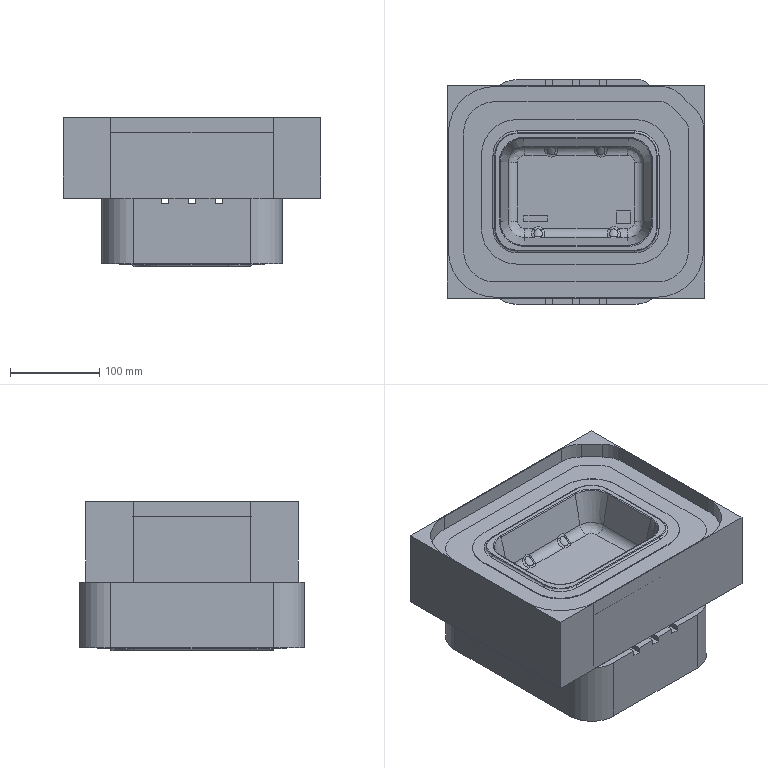NC program | NX | posted with a generic post | part box 287.436 x 251.436 x 167.016 mm
Lines 9781 to 10739 of 118587:
(02 , TOOL : D8)
N19560 M6
N19562 G53
N19564 G17 G0 G90 X-74.765 Y-30.868 S7000 M3 M8
N19566 G43 Z240.5 H0
N19568 Z77.049
N19570 G94 G1 Z76.049 F4500.
N19572 X-78.947
N19574 G3 X-80.547 Y-32.468 R1.6
N19576 G1 Y-33.767
N19578 G3 X-74.266 Y-49.06 R21.919
N19580 X-58.521 Y-55.793 R21.988
N19582 G1 X58.521
N19584 G3 X74.265 Y-49.06 R21.985
N19586 X80.547 Y-33.767 R21.921
N19588 G1 Y-32.476
N19590 G3 X78.947 Y-30.876 R1.6
N19592 G1 X74.765
N19594 Z77.049
N19596 G0 Z93.5
N19598 X43.464 Y-40.046
N19600 Z38.027
N19602 G1 Z37.027
N19604 X44.625 Y-43.436
N19606 G3 X46.657 Y-44.431 R1.6
N19608 G2 X48.138 Y-44.506 R2.
N19610 G3 X48.699 Y-44.666 R1.921
N19612 G2 X50.449 Y-46.65 R2.
N19614 G1 X48.385
N19616 G2 X47.261 Y-46.296 R2.232
N19618 G3 X45.531 Y-45.398 R8.895
N19620 G2 X46.657 Y-44.431 R2.
N19622 G3 X47.652 Y-42.399 R1.6
N19624 G1 X46.678 Y-39.553
N19626 Z38.027
N19628 G0 Z79.049
N19630 X46.793 Y-39.422
N19632 Z37.677
N19634 G1 Z36.677
N19636 X45.177 Y-43.03
N19638 G3 X45.983 Y-45.144 R1.6
N19640 G2 X47.694 Y-46.153 R8.929
N19642 G1 X47.896 Y-46.296
N19644 G3 X48.52 Y-46.517 R1.08
N19646 G1 X50.875
N19648 G3 X52.475 Y-44.917 R1.6
N19650 G1 Y-40.749
N19652 Z37.677
N19654 G0 Z40.027
N19656 X47.461 Y-39.221
N19658 Z37.328
N19660 G1 Z36.328
N19662 X45.678 Y-42.766
N19664 G3 X46.388 Y-44.914 R1.6
N19666 G2 X48.415 Y-46.28 R9.634
N19668 G3 X48.653 Y-46.37 R0.361
N19670 G1 X51.271
N19672 G3 X52.871 Y-44.77 R1.6
N19674 G1 Y-40.601
N19676 Z37.328
N19678 G0 Z39.677
N19680 X48.003 Y-39.005
N19682 Z36.978
N19684 G1 Z35.978
N19686 X46.099 Y-42.475
N19688 G3 X46.732 Y-44.647 R1.6
N19690 G2 X48.81 Y-46.207 R9.174
N19692 G1 X51.593
N19694 G3 X53.193 Y-44.607 R1.6
N19696 G1 Y-40.439
N19698 Z36.978
N19700 G0 Z39.328
N19702 X45.53 Y-38.647
N19704 Z36.629
N19706 G1 Z35.629
N19708 X46.311 Y-42.373
N19710 G3 X48.205 Y-43.611 R1.6
N19712 G2 X49.606 Y-43.831 R2.
N19714 G3 X50.237 Y-44.056 R1.921
N19716 G2 X51.905 Y-46.028 R2.
N19718 G1 X49.081
N19720 G3 X47.011 Y-44.375 R9.539
N19722 G2 X48.205 Y-43.611 R2.
N19724 G3 X49.443 Y-41.717 R1.6
N19726 G1 X48.826 Y-38.772
N19728 Z36.629
N19730 G0 Z38.978
N19732 X44.496 Y-38.001
N19734 Z36.279
N19736 G1 Z35.279
N19738 X46.096 Y-42.468
N19740 G3 X48.142 Y-43.434 R1.6
N19742 G2 X49.857 Y-43.609 R2.
N19744 G3 X50.528 Y-43.861 R1.921
N19746 G2 X52.186 Y-45.832 R2.
N19748 G1 X49.308
N19750 G3 X47.244 Y-44.081 R9.592
N19752 G2 X48.142 Y-43.434 R2.
N19754 G3 X49.108 Y-41.388 R1.6
N19756 G1 X48.094 Y-38.556
N19758 Z36.279
N19760 G0 Z38.629
N19762 X44.067 Y-37.505
N19764 Z35.929
N19766 G1 Z34.929
N19768 X46.989 Y-42.975
N19770 G3 X48.072 Y-43.303 R0.8
N19772 G2 X50.085 Y-43.378 R2.
N19774 G3 X50.78 Y-43.647 R1.921
N19776 G2 X52.432 Y-45.617 R2.
N19778 G1 X49.518
N19780 G3 X47.47 Y-43.797 R9.774
N19782 G2 X48.072 Y-43.303 R2.
N19784 G3 X48.729 Y-41.138 R1.6
N19786 G1 X47.217 Y-38.308
N19788 Z35.929
N19790 G0 Z38.279
N19792 X52.424 Y-38.815
N19794 Z35.58
N19796 G1 Z34.58
N19798 X50.22 Y-43.513
N19800 G3 X47.981 Y-43.182 R1.6
N19802 G2 X50.28 Y-43.121 R2.
N19804 G3 X51.008 Y-43.412 R1.921
N19806 G2 X52.659 Y-45.382 R2.
N19808 G1 X49.691
N19810 G3 X47.659 Y-43.482 R9.75
N19812 G2 X47.981 Y-43.182 R2.
N19814 G3 X48.312 Y-40.943 R1.6
N19816 G1 X45.665 Y-37.378
N19818 Z35.58
N19820 G0 Z37.929
N19822 X50.066 Y-37.705
N19824 Z35.23
N19826 G1 Z34.23
N19828 X47.589 Y-41.031
N19830 G3 X47.916 Y-43.27 R1.6
N19832 X47.745 Y-43.145 R10.561
N19834 G2 X50.415 Y-42.827 R2.
N19836 G3 X51.2 Y-43.155 R1.921
N19838 G2 X52.856 Y-45.125 R2.
N19840 G1 X49.84
N19842 G3 X47.916 Y-43.27 R10.561
N19844 X50.155 Y-42.943 R1.6
N19846 G1 X53.266 Y-38.766
N19848 Z35.23
N19850 G0 Z37.58
N19852 X50.463 Y-37.426
N19854 Z34.881
N19856 G1 Z33.881
N19858 X47.857 Y-40.751
N19860 G3 X48.129 Y-42.998 R1.6
N19862 X47.874 Y-42.804 R10.553
N19864 G2 X50.55 Y-42.526 R2.
N19866 G3 X51.37 Y-42.872 R1.921
N19868 G2 X53.038 Y-44.845 R2.
N19870 G1 X49.965
N19872 G3 X48.129 Y-42.998 R10.553
N19874 X50.375 Y-42.725 R1.6
N19876 G1 X53.639 Y-38.562
N19878 Z34.881
N19880 G0 Z37.23
N19882 X50.071 Y-37.028
N19884 Z34.531
N19886 G1 Z33.531
N19888 X47.67 Y-40.209
N19890 G3 X47.983 Y-42.45 R1.6
N19892 G2 X50.067 Y-44.538 R10.607
N19894 G1 X53.204
N19896 G3 X54.804 Y-42.938 R1.6
N19898 G1 Y-38.769
N19900 Z34.531
N19902 G0 Z36.881
N19904 X50.047 Y-36.563
N19906 Z34.182
N19908 G1 Z33.182
N19910 X47.645 Y-39.711
N19912 G3 X47.946 Y-41.954 R1.6
N19914 G2 X48.955 Y-42.841 R9.628
N19916 G1 X49.077 Y-42.963
N19918 X50.147 Y-44.201
N19920 X53.365
N19922 G3 X54.965 Y-42.601 R1.6
N19924 G1 Y-38.432
N19926 Z34.182
N19928 G0 Z36.531
N19930 X47.442 Y-35.763
N19932 Z33.832
N19934 G1 Z32.832
N19936 X47.658 Y-39.461
N19938 G3 X49.348 Y-40.965 R1.6
N19940 G2 X50.734 Y-41.415 R2.
N19942 G3 X51.752 Y-41.841 R1.921
N19944 G2 X53.544 Y-43.83 R2.
N19946 G1 X50.204
N19948 X49.363 Y-42.841
N19950 G3 X48.025 Y-41.574 R9.605
N19952 G2 X49.348 Y-40.965 R2.
N19954 G3 X50.852 Y-39.274 R1.6
N19956 G1 X50.677 Y-36.27
N19958 Z33.832
N19960 G0 Z79.049
N19962 X37.967 Y-39.545
N19964 Z38.027
N19966 G1 Z37.027
N19968 X36.996 Y-42.393
N19970 G3 X37.995 Y-44.423 R1.6
N19972 G2 X39.124 Y-45.393 R2.
N19974 G3 X37.381 Y-46.296 R8.895
N19976 G2 X36.243 Y-46.65 R2.116
N19978 G1 X34.19
N19980 G2 X35.941 Y-44.665 R2.
N19982 G3 X36.509 Y-44.502 R1.921
N19984 G2 X37.995 Y-44.423 R2.
N19986 G3 X40.026 Y-43.425 R1.6
N19988 G1 X41.176 Y-40.047
N19990 Z38.027
N19992 G0 Z79.049
N19994 X32.166 Y-40.749
N19996 Z37.677
N19998 G1 Z36.677
N20000 Y-44.917
N20002 G3 X33.766 Y-46.517 R1.6
N20004 G1 X36.148
N20006 G3 X36.745 Y-46.296 R1.06
N20008 G1 X37.326 Y-45.899
N20010 G2 X38.691 Y-45.139 R8.929
N20012 G3 X39.5 Y-43.026 R1.6
N20014 G1 X37.885 Y-39.41
N20016 Z37.677
N20018 G0 Z40.027
N20020 X31.785 Y-40.601
N20022 Z37.328
N20024 G1 Z36.328
N20026 Y-44.77
N20028 G3 X33.385 Y-46.37 R1.6
N20030 G1 X35.908
N20032 G3 X36.276 Y-46.232 R0.559
N20034 G2 X38.235 Y-44.917 R9.308
N20036 G3 X38.949 Y-42.77 R1.6
N20038 G1 X37.176 Y-39.227
N20040 Z37.328
N20042 G0 Z39.677
N20044 X42.606 Y-38.719
N20046 Z36.978
N20048 G1 Z35.978
N20050 X38.097 Y-42.3
N20052 G3 X37.839 Y-44.548 R1.6
N20054 G1 X37.911 Y-44.645
N20056 G3 X35.828 Y-46.207 R9.174
N20058 G1 X33.043
N20060 G2 X34.725 Y-44.233 R2.
N20062 G3 X35.327 Y-44.029 R1.921
N20064 G2 X37.839 Y-44.548 R2.
N20066 G3 X35.591 Y-44.29 R1.6
N20068 G1 X33.488 Y-39.588
N20070 Z36.978
N20072 G0 Z39.328
N20074 X32.917 Y-39.475
N20076 Z36.629
N20078 G1 Z35.629
N20080 X35.463 Y-43.801
N20082 G3 X37.653 Y-44.368 R1.6
N20084 X35.561 Y-46.028 R9.641
N20086 G1 X32.732
N20088 G2 X34.4 Y-44.056 R2.
N20090 G3 X35.042 Y-43.825 R1.921
N20092 G2 X37.653 Y-44.368 R2.
N20094 G3 X35.416 Y-44.031 R1.6
N20096 G1 X33.453 Y-39.269
N20098 Z36.629
N20100 G0 Z38.978
N20102 X35.44 Y-38.518
N20104 Z36.279
N20106 G1 Z35.279
N20108 X34.903 Y-41.479
N20110 G3 X36.192 Y-43.339 R1.6
N20112 G2 X37.415 Y-44.081 R2.
N20114 G3 X35.324 Y-45.832 R9.809
N20116 G1 X32.449
N20118 G2 X34.107 Y-43.861 R2.
N20120 G3 X34.786 Y-43.604 R1.921
N20122 G2 X36.192 Y-43.339 R2.
N20124 G3 X38.051 Y-42.051 R1.6
N20126 G1 X38.729 Y-38.319
N20128 Z36.279
N20130 G0 Z38.629
N20132 X36.116 Y-38.26
N20134 Z35.929
N20136 G1 Z34.929
N20138 X35.211 Y-41.13
N20140 G3 X36.255 Y-43.137 R1.6
N20142 G2 X37.205 Y-43.782 R2.
N20144 G3 X35.124 Y-45.617 R9.885
N20146 G1 X32.2
N20148 G2 X33.853 Y-43.647 R2.
N20150 G3 X34.565 Y-43.367 R1.921
N20152 G2 X36.255 Y-43.137 R2.
N20154 G3 X38.262 Y-42.092 R1.6
N20156 G1 X39.66 Y-37.661
N20158 Z35.929
N20160 G0 Z38.279
N20162 X36.826 Y-38.091
N20164 Z35.58
N20166 G1 Z34.58
N20168 X35.563 Y-40.822
N20170 G3 X36.343 Y-42.946 R1.6
N20172 G2 X37.031 Y-43.471 R2.
N20174 G3 X34.952 Y-45.382 R9.992
N20176 G1 X31.979
N20178 G2 X33.632 Y-43.412 R2.
N20180 G3 X34.378 Y-43.108 R1.921
N20182 G2 X36.343 Y-42.946 R2.
N20184 G3 X38.467 Y-42.166 R1.6
N20186 G1 X40.842 Y-37.032
N20188 Z35.58
N20190 G0 Z37.929
N20192 X38.111 Y-37.176
N20194 Z35.23
N20196 G1 Z34.23
N20198 X35.966 Y-40.556
N20200 G3 X36.459 Y-42.764 R1.6
N20202 G2 X36.893 Y-43.136 R2.
N20204 G3 X34.805 Y-45.125 R10.452
N20206 G1 X31.781
N20208 G2 X33.438 Y-43.155 R2.
N20210 G3 X34.225 Y-42.825 R1.921
N20212 G2 X36.459 Y-42.764 R2.
N20214 G3 X37.563 Y-42.518 R0.8
N20216 G1 X41.363 Y-36.532
N20218 Z35.23
N20220 G0 Z37.58
N20222 X39.948 Y-36.26
N20224 Z34.881
N20226 G1 Z33.881
N20228 X36.415 Y-40.363
N20230 G3 X36.584 Y-42.62 R1.6
N20232 G2 X36.765 Y-42.797 R2.
N20234 G3 X34.681 Y-44.845 R10.668
N20236 G1 X31.604
N20238 G2 X33.272 Y-42.872 R2.
N20240 G3 X34.093 Y-42.525 R1.921
N20242 G2 X36.584 Y-42.62 R2.
N20244 G3 X34.327 Y-42.788 R1.6
N20246 G1 X31.813 Y-38.285
N20248 Z34.881
N20250 G0 Z37.23
N20252 X31.05 Y-38.171
N20254 Z34.531
N20256 G1 Z33.531
N20258 X34.277 Y-42.275
N20260 G3 X36.524 Y-42.543 R1.6
N20262 X34.578 Y-44.538 R10.635
N20264 G1 X31.438
N20266 G2 X33.128 Y-42.562 R2.
N20268 G3 X33.981 Y-42.202 R1.921
N20270 G2 X36.649 Y-42.446 R2.
N20272 G1 X36.524 Y-42.543
N20274 G3 X36.792 Y-40.296 R1.6
N20276 G1 X34.252 Y-37.067
N20278 Z34.531
N20280 G0 Z36.881
N20282 X34.042 Y-36.753
N20284 Z34.182
N20286 G1 Z33.182
N20288 X33.78 Y-39.751
N20290 G3 X35.235 Y-41.484 R1.6
N20292 G2 X36.506 Y-42.095 R2.
N20294 G3 X34.495 Y-44.201 R10.045
N20296 G1 X31.276
N20298 G2 X33.002 Y-42.22 R2.
N20300 G3 X33.876 Y-41.865 R1.921
N20302 G2 X35.235 Y-41.484 R2.
N20304 G3 X36.968 Y-40.03 R1.6
N20306 G1 X37.305 Y-36.178
N20308 Z34.182
N20310 G0 Z36.531
N20312 X25.379 Y-39.03
N20314 Z33.832
N20316 G1 Z32.832
N20318 X29.352 Y-42.609
N20320 G3 X31.612 Y-42.491 R1.6
N20322 G2 X32.89 Y-41.841 R2.
N20324 G3 X33.823 Y-41.481 R1.921
N20326 G2 X36.441 Y-41.706 R2.
N20328 G3 X34.437 Y-43.83 R10.091
N20330 G1 X31.098
N20332 G2 X31.612 Y-42.491 R2.
N20334 G3 X31.494 Y-40.232 R1.6
N20336 G1 X29.258 Y-38.218
N20338 Z33.832
N20340 G0 Z79.049
N20342 X-41.179 Y-40.047
N20344 Z38.027
N20346 G1 Z37.027
N20348 X-40.027 Y-43.426
N20350 G3 X-37.997 Y-44.424 R1.6
N20352 G2 X-36.511 Y-44.503 R2.
N20354 G3 X-35.943 Y-44.666 R1.921
N20356 G2 X-34.193 Y-46.65 R2.
N20358 G1 X-36.238
N20360 G2 X-37.385 Y-46.296 R2.226
N20362 G3 X-39.125 Y-45.394 R8.89
N20364 G2 X-37.997 Y-44.424 R2.
N20366 G3 X-36.998 Y-42.394 R1.6
N20368 G1 X-37.969 Y-39.545
N20370 Z38.027
N20372 G0 Z79.049
N20374 X-37.836 Y-39.424
N20376 Z37.677
N20378 G1 Z36.677
N20380 X-39.464 Y-43.036
N20382 G3 X-38.662 Y-45.152 R1.6
N20384 G2 X-37.326 Y-45.898 R8.933
N20386 G1 X-36.745 Y-46.296
N20388 G3 X-36.152 Y-46.517 R1.074
N20390 G1 X-33.776
N20392 G3 X-32.176 Y-44.917 R1.6
N20394 G1 Y-40.749
N20396 Z37.677
N20398 G0 Z40.027
N20400 X-37.264 Y-39.193
N20402 Z37.328
N20404 G1 Z36.328
N20406 X-39.026 Y-42.741
N20408 G3 X-38.305 Y-44.886 R1.6
N20410 G2 X-36.343 Y-46.193 R9.316
N20412 G3 X-35.868 Y-46.37 R0.724
N20414 G1 X-33.381
N20416 G3 X-31.781 Y-44.77 R1.6
N20418 G1 Y-40.601
N20420 Z37.328
N20422 G0 Z39.677
N20424 X-33.48 Y-39.59
N20426 Z36.978
N20428 G1 Z35.978
N20430 X-35.612 Y-44.279
N20432 G3 X-37.86 Y-44.533 R1.6
N20434 G2 X-35.339 Y-44.023 R2.
N20436 G3 X-34.726 Y-44.233 R1.921
N20438 G2 X-33.044 Y-46.207 R2.
N20440 G1 X-35.831
N20442 G3 X-37.94 Y-44.64 R9.507
N20444 G1 X-37.86 Y-44.533
N20446 G3 X-38.114 Y-42.284 R1.6
N20448 G1 X-42.627 Y-38.688
N20450 Z36.978
N20452 G0 Z39.328
N20454 X-33.397 Y-39.301
N20456 Z36.629
N20458 G1 Z35.629
N20460 X-35.383 Y-44.053
N20462 G3 X-37.622 Y-44.379 R1.6
N20464 G2 X-35.034 Y-43.834 R2.
N20466 G3 X-34.408 Y-44.056 R1.921
N20468 G2 X-32.74 Y-46.028 R2.
N20470 G1 X-35.561
N20472 G3 X-37.622 Y-44.379 R9.44
N20474 X-35.43 Y-43.818 R1.6
N20476 G1 X-32.867 Y-39.491
N20478 Z36.629
N20480 G0 Z38.978
N20482 X-38.721 Y-38.315
N20484 Z36.279
N20486 G1 Z35.279
N20488 X-38.043 Y-42.057
N20490 G3 X-36.184 Y-43.346 R1.6
N20492 G2 X-34.784 Y-43.608 R2.
N20494 G3 X-34.11 Y-43.861 R1.921
N20496 G2 X-32.453 Y-45.832 R2.
N20498 G1 X-35.328
N20500 G3 X-37.403 Y-44.082 R9.707
N20502 G2 X-36.184 Y-43.346 R2.
N20504 G3 X-34.895 Y-41.486 R1.6
N20506 G1 X-35.431 Y-38.525
N20508 Z36.279
N20510 G0 Z38.629
N20512 X-39.479 Y-37.649
N20514 Z35.929
N20516 G1 Z34.929
N20518 X-38.236 Y-41.992
N20520 G3 X-36.257 Y-43.09 R1.6
N20522 G2 X-34.593 Y-43.352 R2.
N20524 G3 X-33.858 Y-43.647 R1.921
N20526 G2 X-32.206 Y-45.617 R2.
N20528 G1 X-35.123
N20530 G3 X-37.264 Y-43.758 R11.423
N20532 G2 X-36.257 Y-43.09 R2.
N20534 G3 X-35.159 Y-41.112 R1.6
N20536 G1 X-35.987 Y-38.219
N20538 Z35.929
N20540 G0 Z38.279
N20542 X-40.78 Y-37.038
N20544 Z35.58
N20546 G1 Z34.58
N20548 X-38.44 Y-42.162
N20550 G3 X-36.32 Y-42.953 R1.6
N20552 G2 X-34.371 Y-43.114 R2.
N20554 G3 X-33.632 Y-43.412 R1.921
N20556 G2 X-31.98 Y-45.382 R2.
N20558 G1 X-34.949
N20560 G3 X-37.013 Y-43.477 R9.946
N20562 G2 X-36.32 Y-42.953 R2.
N20564 G3 X-35.529 Y-40.832 R1.6
N20566 G1 X-36.779 Y-38.095
N20568 Z35.58
N20570 G0 Z37.929
N20572 X-41.336 Y-36.541
N20574 Z35.23
N20576 G1 Z34.23
N20578 X-37.526 Y-42.544
N20580 G3 X-36.422 Y-42.791 R0.8
N20582 G2 X-34.207 Y-42.839 R2.
N20584 G3 X-33.439 Y-43.155 R1.921
N20586 G2 X-31.783 Y-45.125 R2.
N20588 G1 X-34.801
N20590 G3 X-36.851 Y-43.157 R10.009
N20592 G2 X-36.422 Y-42.791 R2.
N20594 G3 X-35.929 Y-40.583 R1.6
N20596 G1 X-38.063 Y-37.22
N20598 Z35.23
N20600 G0 Z37.58
N20602 X-31.817 Y-38.283
N20604 Z34.881
N20606 G1 Z33.881
N20608 X-34.311 Y-42.799
N20610 G3 X-36.567 Y-42.622 R1.6
N20612 G2 X-34.087 Y-42.528 R2.
N20614 G3 X-33.272 Y-42.872 R1.921
N20616 G2 X-31.604 Y-44.845 R2.
N20618 G1 X-34.677
N20620 G3 X-36.635 Y-42.918 R9.814
N20622 G1 X-36.763 Y-42.813
N20624 G2 X-36.567 Y-42.622 R2.
N20626 G3 X-36.389 Y-40.366 R1.6
N20628 G1 X-39.878 Y-36.281
N20630 Z34.881
N20632 G0 Z37.23
N20634 X-34.208 Y-37.059
N20636 Z34.531
N20638 G1 Z33.531
N20640 X-36.78 Y-40.312
N20642 G3 X-36.518 Y-42.559 R1.6
N20644 X-36.677 Y-42.436 R11.079
N20646 G2 X-33.992 Y-42.194 R2.
N20648 G3 X-33.128 Y-42.562 R1.921
N20650 G2 X-31.438 Y-44.538 R2.
N20652 G1 X-34.575
N20654 G3 X-36.518 Y-42.559 R11.079
N20656 X-34.27 Y-42.297 R1.6
N20658 G1 X-31.017 Y-38.183
N20660 Z34.531
N20662 G0 Z36.881
N20664 X-33.789 Y-36.759
N20666 Z34.182
N20668 G1 Z33.182
N20670 X-36.512 Y-40.046
N20672 G3 X-36.301 Y-42.298 R1.6
N20674 X-36.594 Y-42.064 R11.041
N20676 G2 X-33.91 Y-41.84 R2.
N20678 G3 X-33.003 Y-42.22 R1.921
N20680 G2 X-31.277 Y-44.201 R2.
N20682 G1 X-34.495
N20684 G3 X-36.301 Y-42.298 R11.041
N20686 X-34.049 Y-42.088 R1.6
N20688 G1 X-30.614 Y-37.944
N20690 Z34.182
N20692 G0 Z36.531
N20694 X-33.329 Y-36.467
N20696 Z33.832
N20698 G1 Z32.832
N20700 X-36.232 Y-39.788
N20702 G3 X-36.081 Y-42.046 R1.6
N20704 X-36.537 Y-41.668 R11.243
N20706 G2 X-33.861 Y-41.453 R2.
N20708 G3 X-32.889 Y-41.841 R1.921
N20710 G2 X-31.098 Y-43.83 R2.
N20712 G1 X-34.438
N20714 G3 X-36.081 Y-42.046 R11.243
N20716 X-33.823 Y-41.895 R1.6
N20718 G1 X-30.156 Y-37.699
N20720 Z33.832
N20722 G0 Z36.182
N20724 X-34.283 Y-35.848
N20726 Z33.482
N20728 G1 Z32.482
N20730 X-36.785 Y-38.979
N20732 G3 X-36.535 Y-41.227 R1.6
N20734 G2 X-34.409 Y-43.419 R12.112
N20736 G1 X34.408
N20738 G2 X36.451 Y-41.274 R10.503
N20740 G3 X36.715 Y-39.026 R1.6
N20742 G1 X34.246 Y-35.9
N20744 Z33.482
N20746 G0 Z35.832
N20748 X-34.316 Y-35.378
N20750 Z33.133
N20752 G1 Z32.133
N20754 X-36.817 Y-38.516
N20756 G3 X-36.563 Y-40.765 R1.6
N20758 G2 X-34.413 Y-42.96 R12.534
N20760 G1 X34.412
N20762 G2 X36.524 Y-40.796 R11.276
N20764 G3 X36.799 Y-38.55 R1.6
N20766 G1 X34.339 Y-35.401
N20768 Z33.133
N20770 G0 Z35.482
N20772 X-34.445 Y-34.846
N20774 Z32.783
N20776 G1 Z31.783
N20778 X-36.928 Y-38.015
N20780 G3 X-36.656 Y-40.261 R1.6
N20782 G2 X-34.445 Y-42.44 R13.701
N20784 G1 X34.446
N20786 G2 X36.608 Y-40.297 R11.852
N20788 G3 X36.909 Y-38.054 R1.6
N20790 G1 X34.478 Y-34.872
N20792 Z32.783
N20794 G0 Z35.133
N20796 X-34.77 Y-34.207
N20798 Z32.434
N20800 G1 Z31.434
N20802 X-37.17 Y-37.449
N20804 G3 X-36.836 Y-39.687 R1.6
N20806 G2 X-34.512 Y-41.841 R14.418
N20808 G1 X34.513
N20810 G2 X36.815 Y-39.707 R13.686
N20812 G3 X37.159 Y-37.471 R1.6
N20814 G1 X34.779 Y-34.224
N20816 Z32.434
N20818 G0 Z34.783
N20820 X30.452 Y-35.182
N20822 Z32.084
N20824 G1 Z31.084
N20826 X31.721 Y-37.998
N20828 G3 X33.837 Y-38.799 R1.6
N20830 G2 X34.112 Y-38.684 R6.
N20832 G3 X34.549 Y-38.443 R1.921
N20834 G2 X37.335 Y-38.855 R2.
N20836 G3 X35.004 Y-40.778 R10.937
N20838 G1 X32.309 Y-40.792
N20840 G2 X33.566 Y-38.925 R2.
N20842 G1 X33.653 Y-38.886
N20844 G2 X33.837 Y-38.799 R6.
N20846 G3 X34.638 Y-36.683 R1.6
N20848 G1 X33.297 Y-33.706
N20850 Z32.084
N20852 G0 Z34.434
N20854 X-37.923 Y-32.38
N20856 Z32.084
N20858 G1 Z31.084
N20860 X-39.505 Y-36.005
N20862 G3 X-38.678 Y-38.111 R1.6
N20864 G2 X-36.739 Y-39.264 R9.036
N20866 X-34.625 Y-41.128 R23.119
N20868 G1 X-10.159 Y-41.005
N20870 G3 X-8.567 Y-39.397 R1.6
N20872 G1 X-8.588 Y-35.228
N20874 Z32.084
N20876 G0 Z79.049
N20878 X-46.676 Y-39.551
N20880 Z38.027
N20882 G1 Z37.027
N20884 X-47.65 Y-42.398
N20886 G3 X-46.654 Y-44.43 R1.6
N20888 G2 X-45.528 Y-45.397 R2.
N20890 G3 X-47.26 Y-46.296 R8.89
N20892 G2 X-48.385 Y-46.65 R2.235
N20894 G1 X-50.449
N20896 G2 X-48.699 Y-44.666 R2.
N20898 G3 X-48.137 Y-44.505 R1.921
N20900 G2 X-46.654 Y-44.43 R2.
N20902 G3 X-44.622 Y-43.434 R1.6
N20904 G1 X-43.464 Y-40.047
N20906 Z38.027
N20908 G0 Z79.049
N20910 X-52.476 Y-40.749
N20912 Z37.677
N20914 G1 Z36.677
N20916 Y-44.917
N20918 G3 X-50.876 Y-46.517 R1.6
N20920 G1 X-48.529
N20922 G3 X-47.871 Y-46.289 R1.061
N20924 G2 X-45.981 Y-45.143 R8.933
N20926 G3 X-45.174 Y-43.029 R1.6
N20928 G1 X-46.789 Y-39.421
N20930 Z37.677
N20932 G0 Z40.027
N20934 X-52.856 Y-40.601
N20936 Z37.328
N20938 G1 Z36.328
N20940 Y-44.77
N20942 G3 X-51.256 Y-46.37 R1.6
N20944 G1 X-48.674
N20946 G3 X-48.418 Y-46.274 R0.388
N20948 G2 X-46.413 Y-44.923 R9.466
N20950 G3 X-45.7 Y-42.775 R1.6
N20952 G1 X-47.478 Y-39.231
N20954 Z37.328
N20956 G0 Z39.677
N20958 X-42.008 Y-38.683
N20960 Z36.978
N20962 G1 Z35.978
N20964 X-46.528 Y-42.283
N20966 G3 X-46.782 Y-44.532 R1.6
N20968 G1 X-46.702 Y-44.64
N20970 G3 X-48.813 Y-46.207 R9.488
N20972 G1 X-51.601
N20974 G2 X-49.919 Y-44.233 R2.
N20976 G3 X-49.305 Y-44.023 R1.921
N20978 G2 X-46.782 Y-44.532 R2.
N20980 G3 X-49.03 Y-44.277 R1.6
N20982 G1 X-51.166 Y-39.59
N20984 Z36.978
N20986 G0 Z39.328
N20988 X-51.69 Y-39.465
N20990 Z36.629
N20992 G1 Z35.629
N20994 X-49.152 Y-43.792
N20996 G3 X-46.963 Y-44.363 R1.6
N20998 X-49.082 Y-46.028 R9.959
N21000 G1 X-51.912
N21002 G2 X-50.244 Y-44.056 R2.
N21004 G3 X-49.591 Y-43.818 R1.921
N21006 G2 X-46.963 Y-44.363 R2.
N21008 G3 X-49.199 Y-44.015 R1.6
N21010 G1 X-51.138 Y-39.243
N21012 Z36.629
N21014 G0 Z38.978
N21016 X-49.198 Y-38.51
N21018 Z36.279
N21020 G1 Z35.279
N21022 X-49.731 Y-41.472
N21024 G3 X-48.44 Y-43.33 R1.6
N21026 G2 X-47.212 Y-44.075 R2.
N21028 G3 X-49.313 Y-45.832 R9.769
N21030 G1 X-52.194
N21032 G2 X-50.536 Y-43.861 R2.
N21034 G3 X-49.85 Y-43.6 R1.921
N21036 G2 X-48.44 Y-43.33 R2.
N21038 G3 X-46.582 Y-42.039 R1.6
N21040 G1 X-45.913 Y-38.324
N21042 Z36.279
N21044 G0 Z38.629
N21046 X-48.573 Y-38.23
N21048 Z35.929
N21050 G1 Z34.929
N21052 X-49.442 Y-41.111
N21054 G3 X-48.372 Y-43.105 R1.6
N21056 G2 X-47.391 Y-43.766 R2.
N21058 G3 X-49.517 Y-45.617 R10.58
N21060 G1 X-52.441
N21062 G2 X-50.788 Y-43.647 R2.
N21064 G3 X-50.057 Y-43.355 R1.921
N21066 G2 X-48.372 Y-43.105 R2.
N21068 G3 X-46.378 Y-42.035 R1.6
N21070 G1 X-45.053 Y-37.64
N21072 Z35.929
N21074 G0 Z38.279
N21076 X-47.78 Y-38.1
N21078 Z35.58
N21080 G1 Z34.58
N21082 X-49.072 Y-40.839
N21084 G3 X-48.308 Y-42.969 R1.6
N21086 G2 X-47.641 Y-43.477 R2.
N21088 G3 X-49.691 Y-45.382 R9.82
N21090 G1 X-52.662
N21092 G2 X-51.01 Y-43.412 R2.
N21094 G3 X-50.275 Y-43.116 R1.921
N21096 G2 X-48.308 Y-42.969 R2.
N21098 G3 X-46.178 Y-42.204 R1.6
N21100 G1 X-43.737 Y-37.027
N21102 Z35.58
N21104 G0 Z37.929
N21106 X-46.434 Y-37.168
N21108 Z35.23
N21110 G1 Z34.23
N21112 X-48.668 Y-40.592
N21114 G3 X-48.202 Y-42.807 R1.6
N21116 G2 X-47.799 Y-43.154 R2.
N21118 G3 X-49.838 Y-45.125 R9.866
N21120 G1 X-52.86
N21122 G2 X-51.203 Y-43.155 R2.
N21124 G3 X-50.437 Y-42.84 R1.921
N21126 G2 X-48.202 Y-42.807 R2.
N21128 G3 X-47.095 Y-42.574 R0.8
N21130 G1 X-43.155 Y-36.535
N21132 Z35.23
N21134 G0 Z37.58
N21136 X-53.573 Y-38.535
N21138 Z34.881
N21140 G1 Z33.881
N21142 X-50.333 Y-42.679
N21144 G3 X-48.087 Y-42.954 R1.6
N21146 X-49.962 Y-44.845 R10.588
N21148 G1 X-53.038
N21150 G2 X-51.369 Y-42.872 R2.
N21152 G3 X-50.552 Y-42.527 R1.921
N21154 G2 X-47.885 Y-42.8 R2.
N21156 G3 X-48.087 Y-42.954 R10.588
N21158 X-47.812 Y-40.708 R1.6
N21160 G1 X-50.385 Y-37.416
N21162 Z34.881
N21164 G0 Z37.23
N21166 X-53.969 Y-38.325
N21168 Z34.531
N21170 G1 Z33.531
N21172 X-50.557 Y-42.471
N21174 G3 X-48.305 Y-42.689 R1.6
N21176 X-50.065 Y-44.538 R10.543
N21178 G1 X-53.204
N21180 G2 X-51.514 Y-42.562 R2.
N21182 G3 X-50.665 Y-42.205 R1.921
N21184 G2 X-48.004 Y-42.451 R2.
N21186 G3 X-48.305 Y-42.689 R10.543
N21188 X-48.087 Y-40.437 R1.6
N21190 G1 X-50.8 Y-37.141
N21192 Z34.531
N21194 G0 Z36.881
N21196 X-54.393 Y-38.112
N21198 Z34.182
N21200 G1 Z33.182
N21202 X-50.785 Y-42.272
N21204 G3 X-48.527 Y-42.433 R1.6
N21206 X-50.146 Y-44.201 R10.433
N21208 G1 X-53.366
N21210 G2 X-51.64 Y-42.22 R2.
N21212 G3 X-50.752 Y-41.855 R1.921
N21214 G2 X-48.102 Y-42.083 R2.
N21216 G3 X-48.527 Y-42.433 R10.433
N21218 X-48.367 Y-40.176 R1.6
N21220 G1 X-51.235 Y-36.868
N21222 Z34.182
N21224 G0 Z36.531
N21226 X-54.845 Y-37.885
N21228 Z33.832
N21230 G1 Z32.832
N21232 X-51.005 Y-42.092
N21234 G3 X-48.744 Y-42.195 R1.6
N21236 X-50.205 Y-43.83 R10.791
N21238 G1 X-53.544
N21240 G2 X-51.752 Y-41.841 R2.
N21242 G3 X-50.796 Y-41.465 R1.921
N21244 G2 X-48.142 Y-41.685 R2.
N21246 G3 X-48.744 Y-42.195 R10.791
N21248 X-48.641 Y-39.935 R1.6
N21250 G1 X-51.691 Y-36.594
N21252 Z33.832
N21254 G0 Z79.716
N21256 X-1.6 Y-106.495
N21258 Z75.048
N21260 G1 Z74.048
N21262 Y-111.993
N21264 G3 X0. Y-113.593 R1.6
N21266 G1 X-90.718
N21268 G2 X-138.518 Y-65.793 R47.8
N21270 G1 Y65.793
N21272 G2 X-90.718 Y113.593 R47.8
N21274 G1 X94.505
N21276 G2 X114.162 Y105.451 R27.8
N21278 G1 X130.376 Y89.237
N21280 G2 X138.518 Y69.58 R27.8
N21282 G1 Y-65.793
N21284 G2 X90.718 Y-113.593 R47.8
N21286 G1 X0.
N21288 G3 X1.6 Y-111.993 R1.6
N21290 G1 Y-106.495
N21292 Z75.048
N21294 G0 Z77.382
N21296 X-1.6
N21298 Z74.715
N21300 G1 Z73.715
N21302 Y-111.993
N21304 G3 X0. Y-113.593 R1.6
N21306 G1 X-90.718
N21308 G2 X-138.518 Y-65.793 R47.8
N21310 G1 Y65.793
N21312 G2 X-90.718 Y113.593 R47.8
N21314 G1 X94.505
N21316 G2 X114.162 Y105.451 R27.8
N21318 G1 X130.376 Y89.237
N21320 G2 X138.518 Y69.58 R27.8
N21322 G1 Y-65.793
N21324 G2 X90.718 Y-113.593 R47.8
N21326 G1 X0.
N21328 G3 X1.6 Y-111.993 R1.6
N21330 G1 Y-106.495
N21332 Z74.715
N21334 G0 Z77.048
N21336 X-1.6 Y-106.053
N21338 Z74.382
N21340 G1 Z73.382
N21342 Y-111.993
N21344 G3 X0. Y-113.593 R1.6
N21346 G1 X-90.718
N21348 G2 X-138.518 Y-65.793 R47.8
N21350 G1 Y65.793
N21352 G2 X-90.718 Y113.593 R47.8
N21354 G1 X94.505
N21356 G2 X114.162 Y105.451 R27.8
N21358 G1 X130.376 Y89.237
N21360 G2 X138.518 Y69.58 R27.8
N21362 G1 Y-65.793
N21364 G2 X90.718 Y-113.593 R47.8
N21366 G1 X0.
N21368 G3 X1.6 Y-111.993 R1.6
N21370 G1 Y-106.053
N21372 Z74.382
N21374 G0 Z77.382
N21376 Y-91.937
N21378 Z75.048
N21380 G1 Z74.048
N21382 Y-86.593
N21384 G3 X0. Y-84.993 R1.6
N21386 G1 X-66.301
N21388 G2 X-109.918 Y-41.376 R43.618
N21390 G1 Y41.376
N21392 G2 X-66.301 Y84.993 R43.617
N21394 G1 X66.301
N21396 G2 X109.918 Y41.376 R43.617
N21398 G1 Y-41.376
N21400 G2 X66.301 Y-84.993 R43.618
N21402 G1 X0.
N21404 G3 X-1.6 Y-86.593 R1.6
N21406 G1 Y-91.937
N21408 Z75.048
N21410 G0 Z77.382
N21412 X1.6 Y-92.071
N21414 Z74.715
N21416 G1 Z73.715
N21418 Y-86.593
N21420 G3 X0. Y-84.993 R1.6
N21422 G1 X-66.301
N21424 G2 X-109.918 Y-41.376 R43.618
N21426 G1 Y41.376
N21428 G2 X-66.301 Y84.993 R43.617
N21430 G1 X66.301
N21432 G2 X109.918 Y41.376 R43.617
N21434 G1 Y-41.376
N21436 G2 X66.301 Y-84.993 R43.618
N21438 G1 X0.
N21440 G3 X-1.6 Y-86.593 R1.6
N21442 G1 Y-92.071
N21444 Z74.715
N21446 G0 Z77.048
N21448 X1.6 Y-92.533
N21450 Z74.382
N21452 G1 Z73.382
N21454 Y-86.593
N21456 G3 X0. Y-84.993 R1.6
N21458 G1 X-66.301
N21460 G2 X-109.918 Y-41.376 R43.618
N21462 G1 Y41.376
N21464 G2 X-66.301 Y84.993 R43.617
N21466 G1 X66.301
N21468 G2 X109.918 Y41.376 R43.617
N21470 G1 Y-41.376